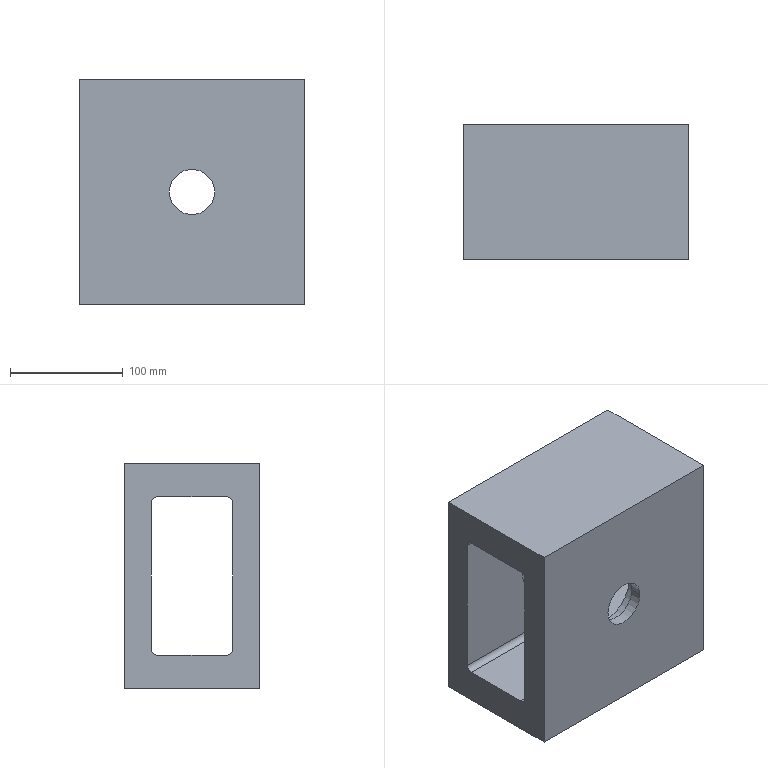Part | SolidWorks | 1 solid | 24 faces | box 200 x 120 x 200 mm | volume 2678625 mm3 | cylinder 12 | plane 12 | commonest cylinder face diameters 10 x4 40 x4 62 x4
STEP:
#1=CARTESIAN_POINT('',(110.359,-52.476,22.5));
#2=VERTEX_POINT('',#1);
#3=CARTESIAN_POINT('',(-89.641,-52.476,22.5));
#4=VERTEX_POINT('',#3);
#5=CARTESIAN_POINT('',(110.359,-52.476,22.5));
#6=DIRECTION('',(-1.,0.,0.));
#7=VECTOR('',#6,1000.);
#8=LINE('',#5,#7);
#9=EDGE_CURVE('',#2,#4,#8,.T.);
#10=ORIENTED_EDGE('',*,*,#9,.F.);
#11=CARTESIAN_POINT('',(110.359,-57.476,27.5));
#12=VERTEX_POINT('',#11);
#13=CARTESIAN_POINT('',(110.359,-57.476,22.5));
#14=DIRECTION('',(1.,0.,0.));
#15=DIRECTION('',(0.,1.,0.));
#16=AXIS2_PLACEMENT_3D('',#13,#14,#15);
#17=CIRCLE('',#16,5.);
#18=EDGE_CURVE('',#2,#12,#17,.T.);
#19=ORIENTED_EDGE('',*,*,#18,.T.);
#20=CARTESIAN_POINT('',(-89.641,-57.476,27.5));
#21=VERTEX_POINT('',#20);
#22=CARTESIAN_POINT('',(-89.641,-57.476,27.5));
#23=DIRECTION('',(1.,0.,0.));
#24=VECTOR('',#23,1000.);
#25=LINE('',#22,#24);
#26=EDGE_CURVE('',#21,#12,#25,.T.);
#27=ORIENTED_EDGE('',*,*,#26,.F.);
#28=CARTESIAN_POINT('',(-89.641,-57.476,22.5));
#29=DIRECTION('',(-1.,0.,0.));
#30=DIRECTION('',(0.,0.,1.));
#31=AXIS2_PLACEMENT_3D('',#28,#29,#30);
#32=CIRCLE('',#31,5.);
#33=EDGE_CURVE('',#21,#4,#32,.T.);
#34=ORIENTED_EDGE('',*,*,#33,.T.);
#35=EDGE_LOOP('',(#10,#19,#27,#34));
#36=FACE_OUTER_BOUND('',#35,.T.);
#37=CARTESIAN_POINT('',(371.079,-57.476,22.5));
#38=DIRECTION('',(-1.,0.,0.));
#39=DIRECTION('',(0.,0.,1.));
#40=AXIS2_PLACEMENT_3D('',#37,#38,#39);
#41=CYLINDRICAL_SURFACE('',#40,5.);
#42=ADVANCED_FACE('',(#36),#41,.F.);
#43=CARTESIAN_POINT('',(110.359,-119.476,27.5));
#44=VERTEX_POINT('',#43);
#45=CARTESIAN_POINT('',(-89.641,-119.476,27.5));
#46=VERTEX_POINT('',#45);
#47=CARTESIAN_POINT('',(110.359,-119.476,27.5));
#48=DIRECTION('',(-1.,0.,0.));
#49=VECTOR('',#48,1000.);
#50=LINE('',#47,#49);
#51=EDGE_CURVE('',#44,#46,#50,.T.);
#52=ORIENTED_EDGE('',*,*,#51,.T.);
#53=CARTESIAN_POINT('',(-89.641,-119.476,27.5));
#54=DIRECTION('',(0.,1.,0.));
#55=VECTOR('',#54,1000.);
#56=LINE('',#53,#55);
#57=EDGE_CURVE('',#46,#21,#56,.T.);
#58=ORIENTED_EDGE('',*,*,#57,.T.);
#59=ORIENTED_EDGE('',*,*,#26,.T.);
#60=CARTESIAN_POINT('',(110.359,-119.476,27.5));
#61=DIRECTION('',(0.,1.,0.));
#62=VECTOR('',#61,1000.);
#63=LINE('',#60,#62);
#64=EDGE_CURVE('',#44,#12,#63,.T.);
#65=ORIENTED_EDGE('',*,*,#64,.F.);
#66=EDGE_LOOP('',(#52,#58,#59,#65));
#67=FACE_OUTER_BOUND('',#66,.T.);
#68=CARTESIAN_POINT('',(0.,-28.476,27.5));
#69=DIRECTION('',(0.,0.,1.));
#70=DIRECTION('',(1.,0.,0.));
#71=AXIS2_PLACEMENT_3D('',#68,#69,#70);
#72=PLANE('',#71);
#73=ADVANCED_FACE('',(#67),#72,.F.);
#74=ORIENTED_EDGE('',*,*,#51,.F.);
#75=CARTESIAN_POINT('',(110.359,-124.476,22.5));
#76=VERTEX_POINT('',#75);
#77=CARTESIAN_POINT('',(110.359,-119.476,22.5));
#78=DIRECTION('',(1.,0.,0.));
#79=DIRECTION('',(0.,0.,1.));
#80=AXIS2_PLACEMENT_3D('',#77,#78,#79);
#81=CIRCLE('',#80,5.);
#82=EDGE_CURVE('',#44,#76,#81,.T.);
#83=ORIENTED_EDGE('',*,*,#82,.T.);
#84=CARTESIAN_POINT('',(-89.641,-124.476,22.5));
#85=VERTEX_POINT('',#84);
#86=CARTESIAN_POINT('',(-89.641,-124.476,22.5));
#87=DIRECTION('',(1.,0.,0.));
#88=VECTOR('',#87,1000.);
#89=LINE('',#86,#88);
#90=EDGE_CURVE('',#85,#76,#89,.T.);
#91=ORIENTED_EDGE('',*,*,#90,.F.);
#92=CARTESIAN_POINT('',(-89.641,-119.476,22.5));
#93=DIRECTION('',(-1.,0.,0.));
#94=DIRECTION('',(0.,-1.,0.));
#95=AXIS2_PLACEMENT_3D('',#92,#93,#94);
#96=CIRCLE('',#95,5.);
#97=EDGE_CURVE('',#85,#46,#96,.T.);
#98=ORIENTED_EDGE('',*,*,#97,.T.);
#99=EDGE_LOOP('',(#74,#83,#91,#98));
#100=FACE_OUTER_BOUND('',#99,.T.);
#101=CARTESIAN_POINT('',(371.079,-119.476,22.5));
#102=DIRECTION('',(-1.,0.,0.));
#103=DIRECTION('',(0.,-1.,0.));
#104=AXIS2_PLACEMENT_3D('',#101,#102,#103);
#105=CYLINDRICAL_SURFACE('',#104,5.);
#106=ADVANCED_FACE('',(#100),#105,.F.);
#107=CARTESIAN_POINT('',(-89.641,-52.476,-107.5));
#108=VERTEX_POINT('',#107);
#109=CARTESIAN_POINT('',(110.359,-52.476,-107.5));
#110=VERTEX_POINT('',#109);
#111=CARTESIAN_POINT('',(-89.641,-52.476,-107.5));
#112=DIRECTION('',(1.,0.,0.));
#113=VECTOR('',#112,1000.);
#114=LINE('',#111,#113);
#115=EDGE_CURVE('',#108,#110,#114,.T.);
#116=ORIENTED_EDGE('',*,*,#115,.F.);
#117=CARTESIAN_POINT('',(-89.641,-57.476,-112.5));
#118=VERTEX_POINT('',#117);
#119=CARTESIAN_POINT('',(-89.641,-57.476,-107.5));
#120=DIRECTION('',(-1.,0.,0.));
#121=DIRECTION('',(0.,1.,0.));
#122=AXIS2_PLACEMENT_3D('',#119,#120,#121);
#123=CIRCLE('',#122,5.);
#124=EDGE_CURVE('',#108,#118,#123,.T.);
#125=ORIENTED_EDGE('',*,*,#124,.T.);
#126=CARTESIAN_POINT('',(110.359,-57.476,-112.5));
#127=VERTEX_POINT('',#126);
#128=CARTESIAN_POINT('',(110.359,-57.476,-112.5));
#129=DIRECTION('',(-1.,0.,0.));
#130=VECTOR('',#129,1000.);
#131=LINE('',#128,#130);
#132=EDGE_CURVE('',#127,#118,#131,.T.);
#133=ORIENTED_EDGE('',*,*,#132,.F.);
#134=CARTESIAN_POINT('',(110.359,-57.476,-107.5));
#135=DIRECTION('',(1.,0.,0.));
#136=DIRECTION('',(0.,0.,-1.));
#137=AXIS2_PLACEMENT_3D('',#134,#135,#136);
#138=CIRCLE('',#137,5.);
#139=EDGE_CURVE('',#127,#110,#138,.T.);
#140=ORIENTED_EDGE('',*,*,#139,.T.);
#141=EDGE_LOOP('',(#116,#125,#133,#140));
#142=FACE_OUTER_BOUND('',#141,.T.);
#143=CARTESIAN_POINT('',(-350.361,-57.476,-107.5));
#144=DIRECTION('',(1.,0.,0.));
#145=DIRECTION('',(0.,0.,-1.));
#146=AXIS2_PLACEMENT_3D('',#143,#144,#145);
#147=CYLINDRICAL_SURFACE('',#146,5.);
#148=ADVANCED_FACE('',(#142),#147,.F.);
#149=CARTESIAN_POINT('',(-89.641,-119.476,-112.5));
#150=VERTEX_POINT('',#149);
#151=CARTESIAN_POINT('',(110.359,-119.476,-112.5));
#152=VERTEX_POINT('',#151);
#153=CARTESIAN_POINT('',(-89.641,-119.476,-112.5));
#154=DIRECTION('',(1.,0.,0.));
#155=VECTOR('',#154,1000.);
#156=LINE('',#153,#155);
#157=EDGE_CURVE('',#150,#152,#156,.T.);
#158=ORIENTED_EDGE('',*,*,#157,.T.);
#159=CARTESIAN_POINT('',(110.359,-57.476,-112.5));
#160=DIRECTION('',(0.,-1.,0.));
#161=VECTOR('',#160,1000.);
#162=LINE('',#159,#161);
#163=EDGE_CURVE('',#127,#152,#162,.T.);
#164=ORIENTED_EDGE('',*,*,#163,.F.);
#165=ORIENTED_EDGE('',*,*,#132,.T.);
#166=CARTESIAN_POINT('',(-89.641,-57.476,-112.5));
#167=DIRECTION('',(0.,-1.,0.));
#168=VECTOR('',#167,1000.);
#169=LINE('',#166,#168);
#170=EDGE_CURVE('',#118,#150,#169,.T.);
#171=ORIENTED_EDGE('',*,*,#170,.T.);
#172=EDGE_LOOP('',(#158,#164,#165,#171));
#173=FACE_OUTER_BOUND('',#172,.T.);
#174=CARTESIAN_POINT('',(0.,-28.476,-112.5));
#175=DIRECTION('',(0.,0.,-1.));
#176=DIRECTION('',(0.,-1.,0.));
#177=AXIS2_PLACEMENT_3D('',#174,#175,#176);
#178=PLANE('',#177);
#179=ADVANCED_FACE('',(#173),#178,.F.);
#180=CARTESIAN_POINT('',(110.359,-124.476,-107.5));
#181=VERTEX_POINT('',#180);
#182=CARTESIAN_POINT('',(-89.641,-124.476,-107.5));
#183=VERTEX_POINT('',#182);
#184=CARTESIAN_POINT('',(110.359,-124.476,-107.5));
#185=DIRECTION('',(-1.,0.,0.));
#186=VECTOR('',#185,1000.);
#187=LINE('',#184,#186);
#188=EDGE_CURVE('',#181,#183,#187,.T.);
#189=ORIENTED_EDGE('',*,*,#188,.F.);
#190=CARTESIAN_POINT('',(110.359,-119.476,-107.5));
#191=DIRECTION('',(1.,0.,0.));
#192=DIRECTION('',(0.,-1.,0.));
#193=AXIS2_PLACEMENT_3D('',#190,#191,#192);
#194=CIRCLE('',#193,5.);
#195=EDGE_CURVE('',#181,#152,#194,.T.);
#196=ORIENTED_EDGE('',*,*,#195,.T.);
#197=ORIENTED_EDGE('',*,*,#157,.F.);
#198=CARTESIAN_POINT('',(-89.641,-119.476,-107.5));
#199=DIRECTION('',(-1.,0.,0.));
#200=DIRECTION('',(0.,0.,-1.));
#201=AXIS2_PLACEMENT_3D('',#198,#199,#200);
#202=CIRCLE('',#201,5.);
#203=EDGE_CURVE('',#150,#183,#202,.T.);
#204=ORIENTED_EDGE('',*,*,#203,.T.);
#205=EDGE_LOOP('',(#189,#196,#197,#204));
#206=FACE_OUTER_BOUND('',#205,.T.);
#207=CARTESIAN_POINT('',(371.079,-119.476,-107.5));
#208=DIRECTION('',(-1.,0.,0.));
#209=DIRECTION('',(0.,0.,-1.));
#210=AXIS2_PLACEMENT_3D('',#207,#208,#209);
#211=CYLINDRICAL_SURFACE('',#210,5.);
#212=ADVANCED_FACE('',(#206),#211,.F.);
#213=CARTESIAN_POINT('',(10.359,-124.476,-11.5));
#214=VERTEX_POINT('',#213);
#215=CARTESIAN_POINT('',(10.359,-124.476,-73.5));
#216=VERTEX_POINT('',#215);
#217=CARTESIAN_POINT('',(10.359,-124.476,-42.5));
#218=DIRECTION('',(0.,1.,0.));
#219=DIRECTION('',(0.,0.,1.));
#220=AXIS2_PLACEMENT_3D('',#217,#218,#219);
#221=CIRCLE('',#220,31.);
#222=EDGE_CURVE('',#214,#216,#221,.T.);
#223=ORIENTED_EDGE('',*,*,#222,.F.);
#224=CARTESIAN_POINT('',(10.359,-124.476,-42.5));
#225=DIRECTION('',(0.,1.,0.));
#226=DIRECTION('',(0.,0.,-1.));
#227=AXIS2_PLACEMENT_3D('',#224,#225,#226);
#228=CIRCLE('',#227,31.);
#229=EDGE_CURVE('',#216,#214,#228,.T.);
#230=ORIENTED_EDGE('',*,*,#229,.F.);
#231=EDGE_LOOP('',(#223,#230));
#232=FACE_BOUND('',#231,.T.);
#233=ORIENTED_EDGE('',*,*,#90,.T.);
#234=CARTESIAN_POINT('',(110.359,-124.476,-107.5));
#235=DIRECTION('',(0.,0.,1.));
#236=VECTOR('',#235,1000.);
#237=LINE('',#234,#236);
#238=EDGE_CURVE('',#181,#76,#237,.T.);
#239=ORIENTED_EDGE('',*,*,#238,.F.);
#240=ORIENTED_EDGE('',*,*,#188,.T.);
#241=CARTESIAN_POINT('',(-89.641,-124.476,-107.5));
#242=DIRECTION('',(0.,0.,1.));
#243=VECTOR('',#242,1000.);
#244=LINE('',#241,#243);
#245=EDGE_CURVE('',#183,#85,#244,.T.);
#246=ORIENTED_EDGE('',*,*,#245,.T.);
#247=EDGE_LOOP('',(#233,#239,#240,#246));
#248=FACE_OUTER_BOUND('',#247,.T.);
#249=CARTESIAN_POINT('',(-49.641,-124.476,57.5));
#250=DIRECTION('',(0.,-1.,0.));
#251=DIRECTION('',(0.,0.,-1.));
#252=AXIS2_PLACEMENT_3D('',#249,#250,#251);
#253=PLANE('',#252);
#254=ADVANCED_FACE('',(#232,#248),#253,.F.);
#255=CARTESIAN_POINT('',(10.359,-138.476,-73.5));
#256=VERTEX_POINT('',#255);
#257=CARTESIAN_POINT('',(10.359,-138.476,-11.5));
#258=VERTEX_POINT('',#257);
#259=CARTESIAN_POINT('',(10.359,-138.476,-42.5));
#260=DIRECTION('',(0.,-1.,0.));
#261=DIRECTION('',(0.,0.,-1.));
#262=AXIS2_PLACEMENT_3D('',#259,#260,#261);
#263=CIRCLE('',#262,31.);
#264=EDGE_CURVE('',#256,#258,#263,.T.);
#265=ORIENTED_EDGE('',*,*,#264,.T.);
#266=CARTESIAN_POINT('',(10.359,-138.476,-11.5));
#267=DIRECTION('',(0.,1.,0.));
#268=VECTOR('',#267,1000.);
#269=LINE('',#266,#268);
#270=EDGE_CURVE('',#258,#214,#269,.T.);
#271=ORIENTED_EDGE('',*,*,#270,.T.);
#272=ORIENTED_EDGE('',*,*,#222,.T.);
#273=CARTESIAN_POINT('',(10.359,-138.476,-73.5));
#274=DIRECTION('',(0.,1.,0.));
#275=VECTOR('',#274,1000.);
#276=LINE('',#273,#275);
#277=EDGE_CURVE('',#256,#216,#276,.T.);
#278=ORIENTED_EDGE('',*,*,#277,.F.);
#279=EDGE_LOOP('',(#265,#271,#272,#278));
#280=FACE_OUTER_BOUND('',#279,.T.);
#281=CARTESIAN_POINT('',(10.359,-124.476,-42.5));
#282=DIRECTION('',(0.,1.,0.));
#283=DIRECTION('',(0.,0.,1.));
#284=AXIS2_PLACEMENT_3D('',#281,#282,#283);
#285=CYLINDRICAL_SURFACE('',#284,31.);
#286=ADVANCED_FACE('',(#280),#285,.F.);
#287=CARTESIAN_POINT('',(10.359,-138.476,-42.5));
#288=DIRECTION('',(0.,-1.,0.));
#289=DIRECTION('',(0.,0.,1.));
#290=AXIS2_PLACEMENT_3D('',#287,#288,#289);
#291=CIRCLE('',#290,31.);
#292=EDGE_CURVE('',#258,#256,#291,.T.);
#293=ORIENTED_EDGE('',*,*,#292,.T.);
#294=ORIENTED_EDGE('',*,*,#277,.T.);
#295=ORIENTED_EDGE('',*,*,#229,.T.);
#296=ORIENTED_EDGE('',*,*,#270,.F.);
#297=EDGE_LOOP('',(#293,#294,#295,#296));
#298=FACE_OUTER_BOUND('',#297,.T.);
#299=CARTESIAN_POINT('',(10.359,-124.476,-42.5));
#300=DIRECTION('',(0.,1.,0.));
#301=DIRECTION('',(0.,0.,1.));
#302=AXIS2_PLACEMENT_3D('',#299,#300,#301);
#303=CYLINDRICAL_SURFACE('',#302,31.);
#304=ADVANCED_FACE('',(#298),#303,.F.);
#305=CARTESIAN_POINT('',(-9.641,-138.476,-42.5));
#306=VERTEX_POINT('',#305);
#307=CARTESIAN_POINT('',(30.359,-138.476,-42.5));
#308=VERTEX_POINT('',#307);
#309=CARTESIAN_POINT('',(10.359,-138.476,-42.5));
#310=DIRECTION('',(0.,1.,0.));
#311=DIRECTION('',(-1.,0.,0.));
#312=AXIS2_PLACEMENT_3D('',#309,#310,#311);
#313=CIRCLE('',#312,20.);
#314=EDGE_CURVE('',#306,#308,#313,.T.);
#315=ORIENTED_EDGE('',*,*,#314,.F.);
#316=CARTESIAN_POINT('',(10.359,-138.476,-42.5));
#317=DIRECTION('',(0.,1.,0.));
#318=DIRECTION('',(1.,0.,0.));
#319=AXIS2_PLACEMENT_3D('',#316,#317,#318);
#320=CIRCLE('',#319,20.);
#321=EDGE_CURVE('',#308,#306,#320,.T.);
#322=ORIENTED_EDGE('',*,*,#321,.F.);
#323=EDGE_LOOP('',(#315,#322));
#324=FACE_BOUND('',#323,.T.);
#325=ORIENTED_EDGE('',*,*,#264,.F.);
#326=ORIENTED_EDGE('',*,*,#292,.F.);
#327=EDGE_LOOP('',(#325,#326));
#328=FACE_OUTER_BOUND('',#327,.T.);
#329=CARTESIAN_POINT('',(0.,-138.476,57.5));
#330=DIRECTION('',(0.,1.,0.));
#331=DIRECTION('',(1.,0.,0.));
#332=AXIS2_PLACEMENT_3D('',#329,#330,#331);
#333=PLANE('',#332);
#334=ADVANCED_FACE('',(#324,#328),#333,.T.);
#335=ORIENTED_EDGE('',*,*,#314,.T.);
#336=CARTESIAN_POINT('',(30.359,-148.476,-42.5));
#337=VERTEX_POINT('',#336);
#338=CARTESIAN_POINT('',(30.359,-138.476,-42.5));
#339=DIRECTION('',(0.,-1.,0.));
#340=VECTOR('',#339,1000.);
#341=LINE('',#338,#340);
#342=EDGE_CURVE('',#308,#337,#341,.T.);
#343=ORIENTED_EDGE('',*,*,#342,.T.);
#344=CARTESIAN_POINT('',(-9.641,-148.476,-42.5));
#345=VERTEX_POINT('',#344);
#346=CARTESIAN_POINT('',(10.359,-148.476,-42.5));
#347=DIRECTION('',(0.,-1.,0.));
#348=DIRECTION('',(1.,0.,0.));
#349=AXIS2_PLACEMENT_3D('',#346,#347,#348);
#350=CIRCLE('',#349,20.);
#351=EDGE_CURVE('',#337,#345,#350,.T.);
#352=ORIENTED_EDGE('',*,*,#351,.T.);
#353=CARTESIAN_POINT('',(-9.641,-138.476,-42.5));
#354=DIRECTION('',(0.,-1.,0.));
#355=VECTOR('',#354,1000.);
#356=LINE('',#353,#355);
#357=EDGE_CURVE('',#306,#345,#356,.T.);
#358=ORIENTED_EDGE('',*,*,#357,.F.);
#359=EDGE_LOOP('',(#335,#343,#352,#358));
#360=FACE_OUTER_BOUND('',#359,.T.);
#361=CARTESIAN_POINT('',(10.359,-148.476,-42.5));
#362=DIRECTION('',(0.,-1.,0.));
#363=DIRECTION('',(1.,0.,0.));
#364=AXIS2_PLACEMENT_3D('',#361,#362,#363);
#365=CYLINDRICAL_SURFACE('',#364,20.);
#366=ADVANCED_FACE('',(#360),#365,.F.);
#367=ORIENTED_EDGE('',*,*,#321,.T.);
#368=ORIENTED_EDGE('',*,*,#357,.T.);
#369=CARTESIAN_POINT('',(10.359,-148.476,-42.5));
#370=DIRECTION('',(0.,-1.,0.));
#371=DIRECTION('',(-1.,0.,0.));
#372=AXIS2_PLACEMENT_3D('',#369,#370,#371);
#373=CIRCLE('',#372,20.);
#374=EDGE_CURVE('',#345,#337,#373,.T.);
#375=ORIENTED_EDGE('',*,*,#374,.T.);
#376=ORIENTED_EDGE('',*,*,#342,.F.);
#377=EDGE_LOOP('',(#367,#368,#375,#376));
#378=FACE_OUTER_BOUND('',#377,.T.);
#379=CARTESIAN_POINT('',(10.359,-148.476,-42.5));
#380=DIRECTION('',(0.,-1.,0.));
#381=DIRECTION('',(1.,0.,0.));
#382=AXIS2_PLACEMENT_3D('',#379,#380,#381);
#383=CYLINDRICAL_SURFACE('',#382,20.);
#384=ADVANCED_FACE('',(#378),#383,.F.);
#385=ORIENTED_EDGE('',*,*,#351,.F.);
#386=ORIENTED_EDGE('',*,*,#374,.F.);
#387=EDGE_LOOP('',(#385,#386));
#388=FACE_BOUND('',#387,.T.);
#389=CARTESIAN_POINT('',(110.359,-148.476,57.5));
#390=VERTEX_POINT('',#389);
#391=CARTESIAN_POINT('',(110.359,-148.476,-142.5));
#392=VERTEX_POINT('',#391);
#393=CARTESIAN_POINT('',(110.359,-148.476,57.5));
#394=DIRECTION('',(0.,0.,-1.));
#395=VECTOR('',#394,1000.);
#396=LINE('',#393,#395);
#397=EDGE_CURVE('',#390,#392,#396,.T.);
#398=ORIENTED_EDGE('',*,*,#397,.F.);
#399=CARTESIAN_POINT('',(-89.641,-148.476,57.5));
#400=VERTEX_POINT('',#399);
#401=CARTESIAN_POINT('',(-89.641,-148.476,57.5));
#402=DIRECTION('',(1.,0.,0.));
#403=VECTOR('',#402,1000.);
#404=LINE('',#401,#403);
#405=EDGE_CURVE('',#400,#390,#404,.T.);
#406=ORIENTED_EDGE('',*,*,#405,.F.);
#407=CARTESIAN_POINT('',(-89.641,-148.476,-142.5));
#408=VERTEX_POINT('',#407);
#409=CARTESIAN_POINT('',(-89.641,-148.476,-142.5));
#410=DIRECTION('',(0.,0.,1.));
#411=VECTOR('',#410,1000.);
#412=LINE('',#409,#411);
#413=EDGE_CURVE('',#408,#400,#412,.T.);
#414=ORIENTED_EDGE('',*,*,#413,.F.);
#415=CARTESIAN_POINT('',(110.359,-148.476,-142.5));
#416=DIRECTION('',(-1.,0.,0.));
#417=VECTOR('',#416,1000.);
#418=LINE('',#415,#417);
#419=EDGE_CURVE('',#392,#408,#418,.T.);
#420=ORIENTED_EDGE('',*,*,#419,.F.);
#421=EDGE_LOOP('',(#398,#406,#414,#420));
#422=FACE_OUTER_BOUND('',#421,.T.);
#423=CARTESIAN_POINT('',(0.,-148.476,0.));
#424=DIRECTION('',(0.,-1.,0.));
#425=DIRECTION('',(0.,0.,-1.));
#426=AXIS2_PLACEMENT_3D('',#423,#424,#425);
#427=PLANE('',#426);
#428=ADVANCED_FACE('',(#388,#422),#427,.T.);
#429=CARTESIAN_POINT('',(10.359,-38.476,-73.5));
#430=VERTEX_POINT('',#429);
#431=CARTESIAN_POINT('',(10.359,-38.476,-11.5));
#432=VERTEX_POINT('',#431);
#433=CARTESIAN_POINT('',(10.359,-38.476,-42.5));
#434=DIRECTION('',(0.,1.,0.));
#435=DIRECTION('',(0.,0.,-1.));
#436=AXIS2_PLACEMENT_3D('',#433,#434,#435);
#437=CIRCLE('',#436,31.);
#438=EDGE_CURVE('',#430,#432,#437,.T.);
#439=ORIENTED_EDGE('',*,*,#438,.T.);
#440=CARTESIAN_POINT('',(10.359,-52.476,-11.5));
#441=VERTEX_POINT('',#440);
#442=CARTESIAN_POINT('',(10.359,-38.476,-11.5));
#443=DIRECTION('',(0.,-1.,0.));
#444=VECTOR('',#443,1000.);
#445=LINE('',#442,#444);
#446=EDGE_CURVE('',#432,#441,#445,.T.);
#447=ORIENTED_EDGE('',*,*,#446,.T.);
#448=CARTESIAN_POINT('',(10.359,-52.476,-73.5));
#449=VERTEX_POINT('',#448);
#450=CARTESIAN_POINT('',(10.359,-52.476,-42.5));
#451=DIRECTION('',(0.,-1.,0.));
#452=DIRECTION('',(0.,0.,1.));
#453=AXIS2_PLACEMENT_3D('',#450,#451,#452);
#454=CIRCLE('',#453,31.);
#455=EDGE_CURVE('',#441,#449,#454,.T.);
#456=ORIENTED_EDGE('',*,*,#455,.T.);
#457=CARTESIAN_POINT('',(10.359,-38.476,-73.5));
#458=DIRECTION('',(0.,-1.,0.));
#459=VECTOR('',#458,1000.);
#460=LINE('',#457,#459);
#461=EDGE_CURVE('',#430,#449,#460,.T.);
#462=ORIENTED_EDGE('',*,*,#461,.F.);
#463=EDGE_LOOP('',(#439,#447,#456,#462));
#464=FACE_OUTER_BOUND('',#463,.T.);
#465=CARTESIAN_POINT('',(10.359,-52.476,-42.5));
#466=DIRECTION('',(0.,-1.,0.));
#467=DIRECTION('',(0.,0.,1.));
#468=AXIS2_PLACEMENT_3D('',#465,#466,#467);
#469=CYLINDRICAL_SURFACE('',#468,31.);
#470=ADVANCED_FACE('',(#464),#469,.F.);
#471=CARTESIAN_POINT('',(10.359,-38.476,-42.5));
#472=DIRECTION('',(0.,1.,0.));
#473=DIRECTION('',(0.,0.,1.));
#474=AXIS2_PLACEMENT_3D('',#471,#472,#473);
#475=CIRCLE('',#474,31.);
#476=EDGE_CURVE('',#432,#430,#475,.T.);
#477=ORIENTED_EDGE('',*,*,#476,.T.);
#478=ORIENTED_EDGE('',*,*,#461,.T.);
#479=CARTESIAN_POINT('',(10.359,-52.476,-42.5));
#480=DIRECTION('',(0.,-1.,0.));
#481=DIRECTION('',(0.,0.,-1.));
#482=AXIS2_PLACEMENT_3D('',#479,#480,#481);
#483=CIRCLE('',#482,31.);
#484=EDGE_CURVE('',#449,#441,#483,.T.);
#485=ORIENTED_EDGE('',*,*,#484,.T.);
#486=ORIENTED_EDGE('',*,*,#446,.F.);
#487=EDGE_LOOP('',(#477,#478,#485,#486));
#488=FACE_OUTER_BOUND('',#487,.T.);
#489=CARTESIAN_POINT('',(10.359,-52.476,-42.5));
#490=DIRECTION('',(0.,-1.,0.));
#491=DIRECTION('',(0.,0.,1.));
#492=AXIS2_PLACEMENT_3D('',#489,#490,#491);
#493=CYLINDRICAL_SURFACE('',#492,31.);
#494=ADVANCED_FACE('',(#488),#493,.F.);
#495=CARTESIAN_POINT('',(30.359,-38.476,-42.5));
#496=VERTEX_POINT('',#495);
#497=CARTESIAN_POINT('',(-9.641,-38.476,-42.5));
#498=VERTEX_POINT('',#497);
#499=CARTESIAN_POINT('',(10.359,-38.476,-42.5));
#500=DIRECTION('',(0.,-1.,0.));
#501=DIRECTION('',(1.,0.,0.));
#502=AXIS2_PLACEMENT_3D('',#499,#500,#501);
#503=CIRCLE('',#502,20.);
#504=EDGE_CURVE('',#496,#498,#503,.T.);
#505=ORIENTED_EDGE('',*,*,#504,.F.);
#506=CARTESIAN_POINT('',(10.359,-38.476,-42.5));
#507=DIRECTION('',(0.,-1.,0.));
#508=DIRECTION('',(-1.,0.,0.));
#509=AXIS2_PLACEMENT_3D('',#506,#507,#508);
#510=CIRCLE('',#509,20.);
#511=EDGE_CURVE('',#498,#496,#510,.T.);
#512=ORIENTED_EDGE('',*,*,#511,.F.);
#513=EDGE_LOOP('',(#505,#512));
#514=FACE_BOUND('',#513,.T.);
#515=ORIENTED_EDGE('',*,*,#438,.F.);
#516=ORIENTED_EDGE('',*,*,#476,.F.);
#517=EDGE_LOOP('',(#515,#516));
#518=FACE_OUTER_BOUND('',#517,.T.);
#519=CARTESIAN_POINT('',(10.359,-38.476,-42.5));
#520=DIRECTION('',(0.,-1.,0.));
#521=DIRECTION('',(0.,0.,-1.));
#522=AXIS2_PLACEMENT_3D('',#519,#520,#521);
#523=PLANE('',#522);
#524=ADVANCED_FACE('',(#514,#518),#523,.T.);
#525=ORIENTED_EDGE('',*,*,#504,.T.);
#526=CARTESIAN_POINT('',(-9.641,-28.476,-42.5));
#527=VERTEX_POINT('',#526);
#528=CARTESIAN_POINT('',(-9.641,-28.476,-42.5));
#529=DIRECTION('',(0.,-1.,0.));
#530=VECTOR('',#529,1000.);
#531=LINE('',#528,#530);
#532=EDGE_CURVE('',#527,#498,#531,.T.);
#533=ORIENTED_EDGE('',*,*,#532,.F.);
#534=CARTESIAN_POINT('',(30.359,-28.476,-42.5));
#535=VERTEX_POINT('',#534);
#536=CARTESIAN_POINT('',(10.359,-28.476,-42.5));
#537=DIRECTION('',(0.,1.,0.));
#538=DIRECTION('',(-1.,0.,0.));
#539=AXIS2_PLACEMENT_3D('',#536,#537,#538);
#540=CIRCLE('',#539,20.);
#541=EDGE_CURVE('',#527,#535,#540,.T.);
#542=ORIENTED_EDGE('',*,*,#541,.T.);
#543=CARTESIAN_POINT('',(30.359,-28.476,-42.5));
#544=DIRECTION('',(0.,-1.,0.));
#545=VECTOR('',#544,1000.);
#546=LINE('',#543,#545);
#547=EDGE_CURVE('',#535,#496,#546,.T.);
#548=ORIENTED_EDGE('',*,*,#547,.T.);
#549=EDGE_LOOP('',(#525,#533,#542,#548));
#550=FACE_OUTER_BOUND('',#549,.T.);
#551=CARTESIAN_POINT('',(10.359,-148.476,-42.5));
#552=DIRECTION('',(0.,-1.,0.));
#553=DIRECTION('',(1.,0.,0.));
#554=AXIS2_PLACEMENT_3D('',#551,#552,#553);
#555=CYLINDRICAL_SURFACE('',#554,20.);
#556=ADVANCED_FACE('',(#550),#555,.F.);
#557=ORIENTED_EDGE('',*,*,#511,.T.);
#558=ORIENTED_EDGE('',*,*,#547,.F.);
#559=CARTESIAN_POINT('',(10.359,-28.476,-42.5));
#560=DIRECTION('',(0.,1.,0.));
#561=DIRECTION('',(1.,0.,0.));
#562=AXIS2_PLACEMENT_3D('',#559,#560,#561);
#563=CIRCLE('',#562,20.);
#564=EDGE_CURVE('',#535,#527,#563,.T.);
#565=ORIENTED_EDGE('',*,*,#564,.T.);
#566=ORIENTED_EDGE('',*,*,#532,.T.);
#567=EDGE_LOOP('',(#557,#558,#565,#566));
#568=FACE_OUTER_BOUND('',#567,.T.);
#569=CARTESIAN_POINT('',(10.359,-148.476,-42.5));
#570=DIRECTION('',(0.,-1.,0.));
#571=DIRECTION('',(1.,0.,0.));
#572=AXIS2_PLACEMENT_3D('',#569,#570,#571);
#573=CYLINDRICAL_SURFACE('',#572,20.);
#574=ADVANCED_FACE('',(#568),#573,.F.);
#575=ORIENTED_EDGE('',*,*,#541,.F.);
#576=ORIENTED_EDGE('',*,*,#564,.F.);
#577=EDGE_LOOP('',(#575,#576));
#578=FACE_BOUND('',#577,.T.);
#579=CARTESIAN_POINT('',(110.359,-28.476,57.5));
#580=VERTEX_POINT('',#579);
#581=CARTESIAN_POINT('',(110.359,-28.476,-142.5));
#582=VERTEX_POINT('',#581);
#583=CARTESIAN_POINT('',(110.359,-28.476,57.5));
#584=DIRECTION('',(0.,0.,-1.));
#585=VECTOR('',#584,1000.);
#586=LINE('',#583,#585);
#587=EDGE_CURVE('',#580,#582,#586,.T.);
#588=ORIENTED_EDGE('',*,*,#587,.T.);
#589=CARTESIAN_POINT('',(-89.641,-28.476,-142.5));
#590=VERTEX_POINT('',#589);
#591=CARTESIAN_POINT('',(110.359,-28.476,-142.5));
#592=DIRECTION('',(-1.,0.,0.));
#593=VECTOR('',#592,1000.);
#594=LINE('',#591,#593);
#595=EDGE_CURVE('',#582,#590,#594,.T.);
#596=ORIENTED_EDGE('',*,*,#595,.T.);
#597=CARTESIAN_POINT('',(-89.641,-28.476,57.5));
#598=VERTEX_POINT('',#597);
#599=CARTESIAN_POINT('',(-89.641,-28.476,-142.5));
#600=DIRECTION('',(0.,0.,1.));
#601=VECTOR('',#600,1000.);
#602=LINE('',#599,#601);
#603=EDGE_CURVE('',#590,#598,#602,.T.);
#604=ORIENTED_EDGE('',*,*,#603,.T.);
#605=CARTESIAN_POINT('',(-89.641,-28.476,57.5));
#606=DIRECTION('',(1.,0.,0.));
#607=VECTOR('',#606,1000.);
#608=LINE('',#605,#607);
#609=EDGE_CURVE('',#598,#580,#608,.T.);
#610=ORIENTED_EDGE('',*,*,#609,.T.);
#611=EDGE_LOOP('',(#588,#596,#604,#610));
#612=FACE_OUTER_BOUND('',#611,.T.);
#613=CARTESIAN_POINT('',(0.,-28.476,0.));
#614=DIRECTION('',(0.,-1.,0.));
#615=DIRECTION('',(0.,0.,-1.));
#616=AXIS2_PLACEMENT_3D('',#613,#614,#615);
#617=PLANE('',#616);
#618=ADVANCED_FACE('',(#578,#612),#617,.F.);
#619=ORIENTED_EDGE('',*,*,#419,.T.);
#620=CARTESIAN_POINT('',(-89.641,-148.476,-142.5));
#621=DIRECTION('',(0.,1.,0.));
#622=VECTOR('',#621,1000.);
#623=LINE('',#620,#622);
#624=EDGE_CURVE('',#408,#590,#623,.T.);
#625=ORIENTED_EDGE('',*,*,#624,.T.);
#626=ORIENTED_EDGE('',*,*,#595,.F.);
#627=CARTESIAN_POINT('',(110.359,-148.476,-142.5));
#628=DIRECTION('',(0.,1.,0.));
#629=VECTOR('',#628,1000.);
#630=LINE('',#627,#629);
#631=EDGE_CURVE('',#392,#582,#630,.T.);
#632=ORIENTED_EDGE('',*,*,#631,.F.);
#633=EDGE_LOOP('',(#619,#625,#626,#632));
#634=FACE_OUTER_BOUND('',#633,.T.);
#635=CARTESIAN_POINT('',(-89.641,-28.476,-142.5));
#636=DIRECTION('',(0.,0.,-1.));
#637=DIRECTION('',(0.,-1.,0.));
#638=AXIS2_PLACEMENT_3D('',#635,#636,#637);
#639=PLANE('',#638);
#640=ADVANCED_FACE('',(#634),#639,.T.);
#641=CARTESIAN_POINT('',(-89.641,-52.476,22.5));
#642=DIRECTION('',(0.,0.,-1.));
#643=VECTOR('',#642,1000.);
#644=LINE('',#641,#643);
#645=EDGE_CURVE('',#4,#108,#644,.T.);
#646=ORIENTED_EDGE('',*,*,#645,.F.);
#647=ORIENTED_EDGE('',*,*,#33,.F.);
#648=ORIENTED_EDGE('',*,*,#57,.F.);
#649=ORIENTED_EDGE('',*,*,#97,.F.);
#650=ORIENTED_EDGE('',*,*,#245,.F.);
#651=ORIENTED_EDGE('',*,*,#203,.F.);
#652=ORIENTED_EDGE('',*,*,#170,.F.);
#653=ORIENTED_EDGE('',*,*,#124,.F.);
#654=EDGE_LOOP('',(#646,#647,#648,#649,#650,#651,#652,#653));
#655=FACE_BOUND('',#654,.T.);
#656=ORIENTED_EDGE('',*,*,#413,.T.);
#657=CARTESIAN_POINT('',(-89.641,-148.476,57.5));
#658=DIRECTION('',(0.,1.,0.));
#659=VECTOR('',#658,1000.);
#660=LINE('',#657,#659);
#661=EDGE_CURVE('',#400,#598,#660,.T.);
#662=ORIENTED_EDGE('',*,*,#661,.T.);
#663=ORIENTED_EDGE('',*,*,#603,.F.);
#664=ORIENTED_EDGE('',*,*,#624,.F.);
#665=EDGE_LOOP('',(#656,#662,#663,#664));
#666=FACE_OUTER_BOUND('',#665,.T.);
#667=CARTESIAN_POINT('',(-89.641,-28.476,57.5));
#668=DIRECTION('',(-1.,0.,0.));
#669=DIRECTION('',(0.,0.,1.));
#670=AXIS2_PLACEMENT_3D('',#667,#668,#669);
#671=PLANE('',#670);
#672=ADVANCED_FACE('',(#655,#666),#671,.T.);
#673=ORIENTED_EDGE('',*,*,#405,.T.);
#674=CARTESIAN_POINT('',(110.359,-148.476,57.5));
#675=DIRECTION('',(0.,1.,0.));
#676=VECTOR('',#675,1000.);
#677=LINE('',#674,#676);
#678=EDGE_CURVE('',#390,#580,#677,.T.);
#679=ORIENTED_EDGE('',*,*,#678,.T.);
#680=ORIENTED_EDGE('',*,*,#609,.F.);
#681=ORIENTED_EDGE('',*,*,#661,.F.);
#682=EDGE_LOOP('',(#673,#679,#680,#681));
#683=FACE_OUTER_BOUND('',#682,.T.);
#684=CARTESIAN_POINT('',(110.359,-28.476,57.5));
#685=DIRECTION('',(0.,0.,1.));
#686=DIRECTION('',(1.,0.,0.));
#687=AXIS2_PLACEMENT_3D('',#684,#685,#686);
#688=PLANE('',#687);
#689=ADVANCED_FACE('',(#683),#688,.T.);
#690=ORIENTED_EDGE('',*,*,#64,.T.);
#691=ORIENTED_EDGE('',*,*,#18,.F.);
#692=CARTESIAN_POINT('',(110.359,-52.476,22.5));
#693=DIRECTION('',(0.,0.,-1.));
#694=VECTOR('',#693,1000.);
#695=LINE('',#692,#694);
#696=EDGE_CURVE('',#2,#110,#695,.T.);
#697=ORIENTED_EDGE('',*,*,#696,.T.);
#698=ORIENTED_EDGE('',*,*,#139,.F.);
#699=ORIENTED_EDGE('',*,*,#163,.T.);
#700=ORIENTED_EDGE('',*,*,#195,.F.);
#701=ORIENTED_EDGE('',*,*,#238,.T.);
#702=ORIENTED_EDGE('',*,*,#82,.F.);
#703=EDGE_LOOP('',(#690,#691,#697,#698,#699,#700,#701,#702));
#704=FACE_BOUND('',#703,.T.);
#705=ORIENTED_EDGE('',*,*,#397,.T.);
#706=ORIENTED_EDGE('',*,*,#631,.T.);
#707=ORIENTED_EDGE('',*,*,#587,.F.);
#708=ORIENTED_EDGE('',*,*,#678,.F.);
#709=EDGE_LOOP('',(#705,#706,#707,#708));
#710=FACE_OUTER_BOUND('',#709,.T.);
#711=CARTESIAN_POINT('',(110.359,-28.476,-142.5));
#712=DIRECTION('',(1.,0.,0.));
#713=DIRECTION('',(0.,1.,0.));
#714=AXIS2_PLACEMENT_3D('',#711,#712,#713);
#715=PLANE('',#714);
#716=ADVANCED_FACE('',(#704,#710),#715,.T.);
#717=ORIENTED_EDGE('',*,*,#455,.F.);
#718=ORIENTED_EDGE('',*,*,#484,.F.);
#719=EDGE_LOOP('',(#717,#718));
#720=FACE_BOUND('',#719,.T.);
#721=ORIENTED_EDGE('',*,*,#9,.T.);
#722=ORIENTED_EDGE('',*,*,#645,.T.);
#723=ORIENTED_EDGE('',*,*,#115,.T.);
#724=ORIENTED_EDGE('',*,*,#696,.F.);
#725=EDGE_LOOP('',(#721,#722,#723,#724));
#726=FACE_OUTER_BOUND('',#725,.T.);
#727=CARTESIAN_POINT('',(70.359,-52.476,57.5));
#728=DIRECTION('',(0.,1.,0.));
#729=DIRECTION('',(1.,0.,0.));
#730=AXIS2_PLACEMENT_3D('',#727,#728,#729);
#731=PLANE('',#730);
#732=ADVANCED_FACE('',(#720,#726),#731,.F.);
#733=CLOSED_SHELL('',(#42,#73,#106,#148,#179,#212,#254,#286,#304,#334,#366,#384,#428,#470,#494,#524,#556,#574,#618,#640,#672,#689,#716,#732));
#734=MANIFOLD_SOLID_BREP('',#733);
#735=CARTESIAN_POINT('',(0.,0.,0.));
#736=DIRECTION('',(0.,0.,1.));
#737=DIRECTION('',(1.,0.,0.));
#738=AXIS2_PLACEMENT_3D('',#735,#736,#737);
#739=(LENGTH_UNIT()NAMED_UNIT(*)SI_UNIT(.MILLI.,.METRE.));
#740=UNCERTAINTY_MEASURE_WITH_UNIT(LENGTH_MEASURE(0.00001),#739,'','');
#741=(NAMED_UNIT(*)PLANE_ANGLE_UNIT()SI_UNIT($,.RADIAN.));
#742=(NAMED_UNIT(*)SI_UNIT($,.STERADIAN.)SOLID_ANGLE_UNIT());
#743=(GEOMETRIC_REPRESENTATION_CONTEXT(3)GLOBAL_UNCERTAINTY_ASSIGNED_CONTEXT((#740))GLOBAL_UNIT_ASSIGNED_CONTEXT((#739,#741,#742))REPRESENTATION_CONTEXT('',''));
#744=ADVANCED_BREP_SHAPE_REPRESENTATION('',(#734,#738),#743);